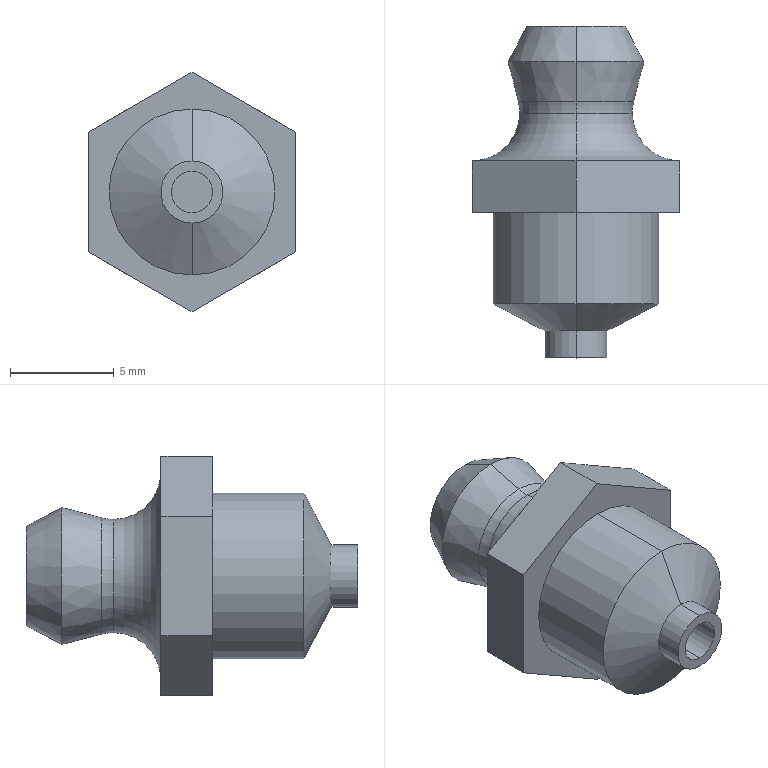Part | STEP file | Straight Grease Fitting JB/T7940.1-1995 8 | 1 solid | 35 faces | box 10 x 16 x 11.547 mm | volume 627.523 mm3 | plane 17 | cylinder 8 | cone 6 | torus 4 | commonest cylinder face diameters 2 x4 3 x2 8 x2